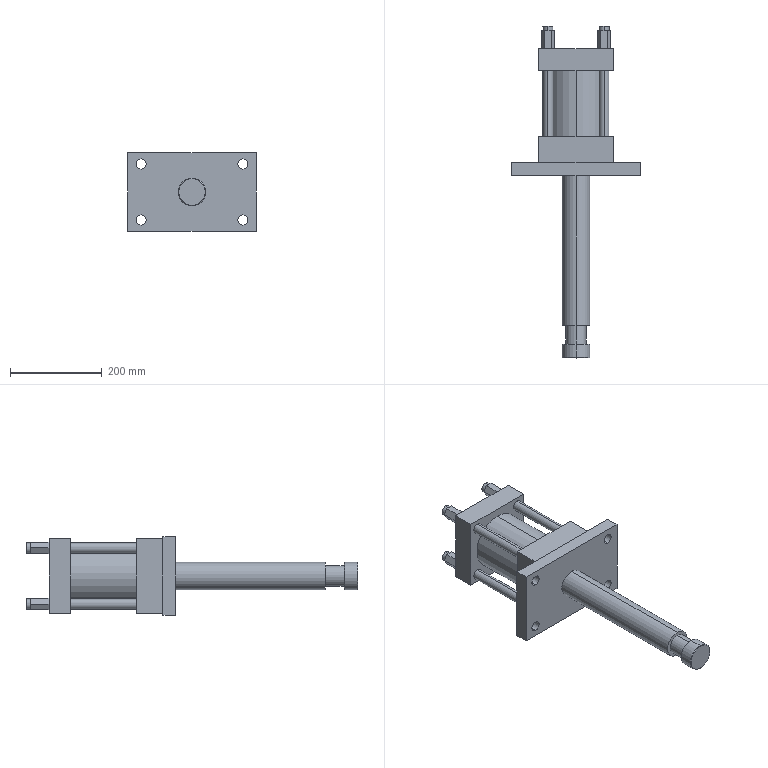Part | SolidWorks | features BaseBody 1 | 1 solid | 94 faces | box 280 x 722.65 x 170 mm | volume 7160038 mm3 | plane 54 | cylinder 36 | cone 4 | commonest cylinder face diameters 22 x28 60 x4 44 x2 125 x2